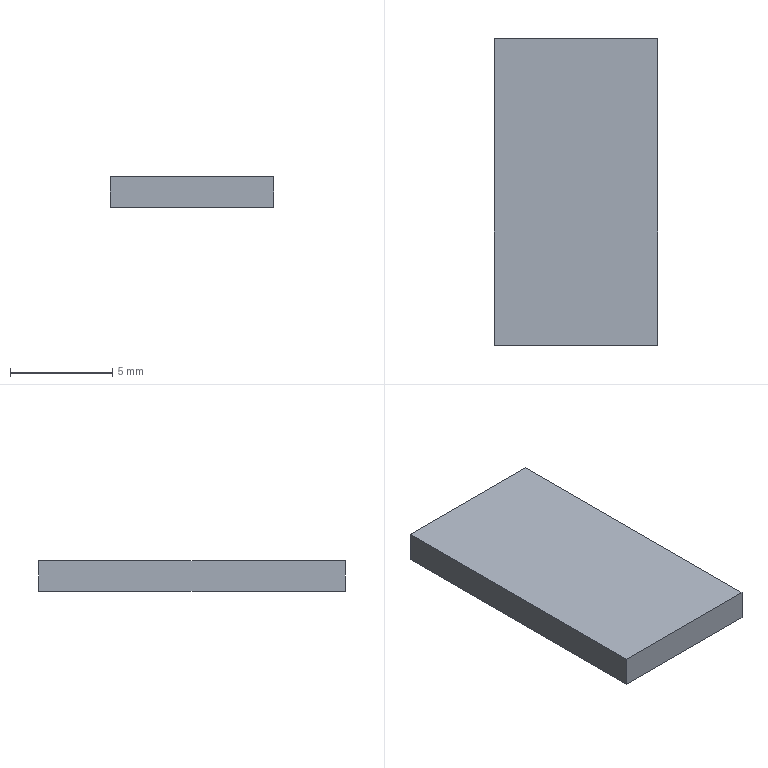Part | STEP file | T2x15x8 Rubber strip-dddeger_compressed | 1 solid | 6 faces | box 8 x 15 x 1.5 mm | volume 180 mm3 | plane 6
STEP:
#1=CARTESIAN_POINT('',(0.,0.,0.));
#2=DIRECTION('',(0.,0.,1.));
#3=DIRECTION('',(1.,0.,0.));
#4=AXIS2_PLACEMENT_3D('',#1,#2,#3);
#5=CARTESIAN_POINT('',(-629.155,-97.655,0.));
#6=VERTEX_POINT('',#5);
#7=CARTESIAN_POINT('',(-629.155,-82.655,0.));
#8=VERTEX_POINT('',#7);
#9=CARTESIAN_POINT('',(-629.155,-82.655,0.));
#10=DIRECTION('',(0.,1.,0.));
#11=VECTOR('',#10,1.);
#12=LINE('',#9,#11);
#13=CARTESIAN_POINT('',(-629.155,-82.655,1.5));
#14=DIRECTION('',(-1.,0.,0.));
#15=DIRECTION('',(0.,0.,1.));
#16=AXIS2_PLACEMENT_3D('',#13,#14,#15);
#17=PLANE('',#16);
#18=CARTESIAN_POINT('',(-1.5,0.));
#19=DIRECTION('',(0.,1.));
#20=VECTOR('',#19,1.);
#21=LINE('',#18,#20);
#22=(GEOMETRIC_REPRESENTATION_CONTEXT(2)PARAMETRIC_REPRESENTATION_CONTEXT()REPRESENTATION_CONTEXT('',''));
#23=DEFINITIONAL_REPRESENTATION('',(#21),#22);
#24=PCURVE('',#17,#23);
#25=CARTESIAN_POINT('',(0.,0.,0.));
#26=DIRECTION('',(0.,0.,-1.));
#27=DIRECTION('',(-1.,0.,0.));
#28=AXIS2_PLACEMENT_3D('',#25,#26,#27);
#29=PLANE('',#28);
#30=CARTESIAN_POINT('',(629.155,-82.655));
#31=DIRECTION('',(0.,1.));
#32=VECTOR('',#31,1.);
#33=LINE('',#30,#32);
#34=(GEOMETRIC_REPRESENTATION_CONTEXT(2)PARAMETRIC_REPRESENTATION_CONTEXT()REPRESENTATION_CONTEXT('',''));
#35=DEFINITIONAL_REPRESENTATION('',(#33),#34);
#36=PCURVE('',#29,#35);
#37=SURFACE_CURVE('',#12,(#24,#36),.PCURVE_S1.);
#38=EDGE_CURVE('',#6,#8,#37,.T.);
#39=ORIENTED_EDGE('',*,*,#38,.T.);
#40=CARTESIAN_POINT('',(-629.155,-82.655,1.5));
#41=VERTEX_POINT('',#40);
#42=CARTESIAN_POINT('',(-629.155,-82.655,1.5));
#43=DIRECTION('',(0.,0.,-1.));
#44=VECTOR('',#43,1.);
#45=LINE('',#42,#44);
#46=CARTESIAN_POINT('',(0.,0.));
#47=DIRECTION('',(-1.,0.));
#48=VECTOR('',#47,1.);
#49=LINE('',#46,#48);
#50=(GEOMETRIC_REPRESENTATION_CONTEXT(2)PARAMETRIC_REPRESENTATION_CONTEXT()REPRESENTATION_CONTEXT('',''));
#51=DEFINITIONAL_REPRESENTATION('',(#49),#50);
#52=PCURVE('',#17,#51);
#53=CARTESIAN_POINT('',(-629.155,-82.655,1.5));
#54=DIRECTION('',(0.,-1.,0.));
#55=DIRECTION('',(0.,0.,-1.));
#56=AXIS2_PLACEMENT_3D('',#53,#54,#55);
#57=PLANE('',#56);
#58=CARTESIAN_POINT('',(0.,0.));
#59=DIRECTION('',(1.,0.));
#60=VECTOR('',#59,1.);
#61=LINE('',#58,#60);
#62=(GEOMETRIC_REPRESENTATION_CONTEXT(2)PARAMETRIC_REPRESENTATION_CONTEXT()REPRESENTATION_CONTEXT('',''));
#63=DEFINITIONAL_REPRESENTATION('',(#61),#62);
#64=PCURVE('',#57,#63);
#65=SURFACE_CURVE('',#45,(#52,#64),.PCURVE_S1.);
#66=EDGE_CURVE('',#41,#8,#65,.T.);
#67=ORIENTED_EDGE('',*,*,#66,.F.);
#68=CARTESIAN_POINT('',(-629.155,-97.655,1.5));
#69=VERTEX_POINT('',#68);
#70=CARTESIAN_POINT('',(-629.155,-82.655,1.5));
#71=DIRECTION('',(0.,1.,0.));
#72=VECTOR('',#71,1.);
#73=LINE('',#70,#72);
#74=CARTESIAN_POINT('',(0.,0.));
#75=DIRECTION('',(0.,1.));
#76=VECTOR('',#75,1.);
#77=LINE('',#74,#76);
#78=(GEOMETRIC_REPRESENTATION_CONTEXT(2)PARAMETRIC_REPRESENTATION_CONTEXT()REPRESENTATION_CONTEXT('',''));
#79=DEFINITIONAL_REPRESENTATION('',(#77),#78);
#80=PCURVE('',#17,#79);
#81=CARTESIAN_POINT('',(0.,0.,1.5));
#82=DIRECTION('',(0.,0.,-1.));
#83=DIRECTION('',(-1.,0.,0.));
#84=AXIS2_PLACEMENT_3D('',#81,#82,#83);
#85=PLANE('',#84);
#86=CARTESIAN_POINT('',(629.155,-82.655));
#87=DIRECTION('',(0.,1.));
#88=VECTOR('',#87,1.);
#89=LINE('',#86,#88);
#90=(GEOMETRIC_REPRESENTATION_CONTEXT(2)PARAMETRIC_REPRESENTATION_CONTEXT()REPRESENTATION_CONTEXT('',''));
#91=DEFINITIONAL_REPRESENTATION('',(#89),#90);
#92=PCURVE('',#85,#91);
#93=SURFACE_CURVE('',#73,(#80,#92),.PCURVE_S1.);
#94=EDGE_CURVE('',#69,#41,#93,.T.);
#95=ORIENTED_EDGE('',*,*,#94,.F.);
#96=CARTESIAN_POINT('',(-629.155,-97.655,1.5));
#97=DIRECTION('',(0.,0.,-1.));
#98=VECTOR('',#97,1.);
#99=LINE('',#96,#98);
#100=CARTESIAN_POINT('',(0.,-15.));
#101=DIRECTION('',(-1.,0.));
#102=VECTOR('',#101,1.);
#103=LINE('',#100,#102);
#104=(GEOMETRIC_REPRESENTATION_CONTEXT(2)PARAMETRIC_REPRESENTATION_CONTEXT()REPRESENTATION_CONTEXT('',''));
#105=DEFINITIONAL_REPRESENTATION('',(#103),#104);
#106=PCURVE('',#17,#105);
#107=CARTESIAN_POINT('',(-629.155,-97.655,1.5));
#108=DIRECTION('',(0.,1.,0.));
#109=DIRECTION('',(0.,0.,1.));
#110=AXIS2_PLACEMENT_3D('',#107,#108,#109);
#111=PLANE('',#110);
#112=CARTESIAN_POINT('',(0.,0.));
#113=DIRECTION('',(-1.,0.));
#114=VECTOR('',#113,1.);
#115=LINE('',#112,#114);
#116=(GEOMETRIC_REPRESENTATION_CONTEXT(2)PARAMETRIC_REPRESENTATION_CONTEXT()REPRESENTATION_CONTEXT('',''));
#117=DEFINITIONAL_REPRESENTATION('',(#115),#116);
#118=PCURVE('',#111,#117);
#119=SURFACE_CURVE('',#99,(#106,#118),.PCURVE_S1.);
#120=EDGE_CURVE('',#69,#6,#119,.T.);
#121=ORIENTED_EDGE('',*,*,#120,.T.);
#122=EDGE_LOOP('',(#39,#67,#95,#121));
#123=FACE_BOUND('',#122,.T.);
#124=ADVANCED_FACE('',(#123),#17,.F.);
#125=CARTESIAN_POINT('',(-637.155,-82.655,0.));
#126=VERTEX_POINT('',#125);
#127=CARTESIAN_POINT('',(-629.155,-82.655,0.));
#128=DIRECTION('',(-1.,0.,0.));
#129=VECTOR('',#128,1.);
#130=LINE('',#127,#129);
#131=CARTESIAN_POINT('',(1.5,0.));
#132=DIRECTION('',(0.,-1.));
#133=VECTOR('',#132,1.);
#134=LINE('',#131,#133);
#135=(GEOMETRIC_REPRESENTATION_CONTEXT(2)PARAMETRIC_REPRESENTATION_CONTEXT()REPRESENTATION_CONTEXT('',''));
#136=DEFINITIONAL_REPRESENTATION('',(#134),#135);
#137=PCURVE('',#57,#136);
#138=CARTESIAN_POINT('',(629.155,-82.655));
#139=DIRECTION('',(1.,0.));
#140=VECTOR('',#139,1.);
#141=LINE('',#138,#140);
#142=(GEOMETRIC_REPRESENTATION_CONTEXT(2)PARAMETRIC_REPRESENTATION_CONTEXT()REPRESENTATION_CONTEXT('',''));
#143=DEFINITIONAL_REPRESENTATION('',(#141),#142);
#144=PCURVE('',#29,#143);
#145=SURFACE_CURVE('',#130,(#137,#144),.PCURVE_S1.);
#146=EDGE_CURVE('',#8,#126,#145,.T.);
#147=ORIENTED_EDGE('',*,*,#146,.T.);
#148=CARTESIAN_POINT('',(-637.155,-82.655,1.5));
#149=VERTEX_POINT('',#148);
#150=CARTESIAN_POINT('',(-637.155,-82.655,1.5));
#151=DIRECTION('',(0.,0.,-1.));
#152=VECTOR('',#151,1.);
#153=LINE('',#150,#152);
#154=CARTESIAN_POINT('',(0.,-8.));
#155=DIRECTION('',(1.,0.));
#156=VECTOR('',#155,1.);
#157=LINE('',#154,#156);
#158=(GEOMETRIC_REPRESENTATION_CONTEXT(2)PARAMETRIC_REPRESENTATION_CONTEXT()REPRESENTATION_CONTEXT('',''));
#159=DEFINITIONAL_REPRESENTATION('',(#157),#158);
#160=PCURVE('',#57,#159);
#161=CARTESIAN_POINT('',(-637.155,-82.655,1.5));
#162=DIRECTION('',(1.,0.,0.));
#163=DIRECTION('',(0.,0.,-1.));
#164=AXIS2_PLACEMENT_3D('',#161,#162,#163);
#165=PLANE('',#164);
#166=CARTESIAN_POINT('',(0.,0.));
#167=DIRECTION('',(1.,0.));
#168=VECTOR('',#167,1.);
#169=LINE('',#166,#168);
#170=(GEOMETRIC_REPRESENTATION_CONTEXT(2)PARAMETRIC_REPRESENTATION_CONTEXT()REPRESENTATION_CONTEXT('',''));
#171=DEFINITIONAL_REPRESENTATION('',(#169),#170);
#172=PCURVE('',#165,#171);
#173=SURFACE_CURVE('',#153,(#160,#172),.PCURVE_S1.);
#174=EDGE_CURVE('',#149,#126,#173,.T.);
#175=ORIENTED_EDGE('',*,*,#174,.F.);
#176=CARTESIAN_POINT('',(-629.155,-82.655,1.5));
#177=DIRECTION('',(-1.,0.,0.));
#178=VECTOR('',#177,1.);
#179=LINE('',#176,#178);
#180=CARTESIAN_POINT('',(0.,0.));
#181=DIRECTION('',(0.,-1.));
#182=VECTOR('',#181,1.);
#183=LINE('',#180,#182);
#184=(GEOMETRIC_REPRESENTATION_CONTEXT(2)PARAMETRIC_REPRESENTATION_CONTEXT()REPRESENTATION_CONTEXT('',''));
#185=DEFINITIONAL_REPRESENTATION('',(#183),#184);
#186=PCURVE('',#57,#185);
#187=CARTESIAN_POINT('',(629.155,-82.655));
#188=DIRECTION('',(1.,0.));
#189=VECTOR('',#188,1.);
#190=LINE('',#187,#189);
#191=(GEOMETRIC_REPRESENTATION_CONTEXT(2)PARAMETRIC_REPRESENTATION_CONTEXT()REPRESENTATION_CONTEXT('',''));
#192=DEFINITIONAL_REPRESENTATION('',(#190),#191);
#193=PCURVE('',#85,#192);
#194=SURFACE_CURVE('',#179,(#186,#193),.PCURVE_S1.);
#195=EDGE_CURVE('',#41,#149,#194,.T.);
#196=ORIENTED_EDGE('',*,*,#195,.F.);
#197=ORIENTED_EDGE('',*,*,#66,.T.);
#198=EDGE_LOOP('',(#147,#175,#196,#197));
#199=FACE_BOUND('',#198,.T.);
#200=ADVANCED_FACE('',(#199),#57,.F.);
#201=CARTESIAN_POINT('',(-637.155,-97.655,0.));
#202=VERTEX_POINT('',#201);
#203=CARTESIAN_POINT('',(-637.155,-82.655,0.));
#204=DIRECTION('',(0.,-1.,0.));
#205=VECTOR('',#204,1.);
#206=LINE('',#203,#205);
#207=CARTESIAN_POINT('',(1.5,0.));
#208=DIRECTION('',(0.,-1.));
#209=VECTOR('',#208,1.);
#210=LINE('',#207,#209);
#211=(GEOMETRIC_REPRESENTATION_CONTEXT(2)PARAMETRIC_REPRESENTATION_CONTEXT()REPRESENTATION_CONTEXT('',''));
#212=DEFINITIONAL_REPRESENTATION('',(#210),#211);
#213=PCURVE('',#165,#212);
#214=CARTESIAN_POINT('',(637.155,-82.655));
#215=DIRECTION('',(0.,-1.));
#216=VECTOR('',#215,1.);
#217=LINE('',#214,#216);
#218=(GEOMETRIC_REPRESENTATION_CONTEXT(2)PARAMETRIC_REPRESENTATION_CONTEXT()REPRESENTATION_CONTEXT('',''));
#219=DEFINITIONAL_REPRESENTATION('',(#217),#218);
#220=PCURVE('',#29,#219);
#221=SURFACE_CURVE('',#206,(#213,#220),.PCURVE_S1.);
#222=EDGE_CURVE('',#126,#202,#221,.T.);
#223=ORIENTED_EDGE('',*,*,#222,.T.);
#224=CARTESIAN_POINT('',(-637.155,-97.655,1.5));
#225=VERTEX_POINT('',#224);
#226=CARTESIAN_POINT('',(-637.155,-97.655,1.5));
#227=DIRECTION('',(0.,0.,-1.));
#228=VECTOR('',#227,1.);
#229=LINE('',#226,#228);
#230=CARTESIAN_POINT('',(0.,-15.));
#231=DIRECTION('',(1.,0.));
#232=VECTOR('',#231,1.);
#233=LINE('',#230,#232);
#234=(GEOMETRIC_REPRESENTATION_CONTEXT(2)PARAMETRIC_REPRESENTATION_CONTEXT()REPRESENTATION_CONTEXT('',''));
#235=DEFINITIONAL_REPRESENTATION('',(#233),#234);
#236=PCURVE('',#165,#235);
#237=CARTESIAN_POINT('',(0.,-8.));
#238=DIRECTION('',(-1.,0.));
#239=VECTOR('',#238,1.);
#240=LINE('',#237,#239);
#241=(GEOMETRIC_REPRESENTATION_CONTEXT(2)PARAMETRIC_REPRESENTATION_CONTEXT()REPRESENTATION_CONTEXT('',''));
#242=DEFINITIONAL_REPRESENTATION('',(#240),#241);
#243=PCURVE('',#111,#242);
#244=SURFACE_CURVE('',#229,(#236,#243),.PCURVE_S1.);
#245=EDGE_CURVE('',#225,#202,#244,.T.);
#246=ORIENTED_EDGE('',*,*,#245,.F.);
#247=CARTESIAN_POINT('',(-637.155,-82.655,1.5));
#248=DIRECTION('',(0.,-1.,0.));
#249=VECTOR('',#248,1.);
#250=LINE('',#247,#249);
#251=CARTESIAN_POINT('',(0.,0.));
#252=DIRECTION('',(0.,-1.));
#253=VECTOR('',#252,1.);
#254=LINE('',#251,#253);
#255=(GEOMETRIC_REPRESENTATION_CONTEXT(2)PARAMETRIC_REPRESENTATION_CONTEXT()REPRESENTATION_CONTEXT('',''));
#256=DEFINITIONAL_REPRESENTATION('',(#254),#255);
#257=PCURVE('',#165,#256);
#258=CARTESIAN_POINT('',(637.155,-82.655));
#259=DIRECTION('',(0.,-1.));
#260=VECTOR('',#259,1.);
#261=LINE('',#258,#260);
#262=(GEOMETRIC_REPRESENTATION_CONTEXT(2)PARAMETRIC_REPRESENTATION_CONTEXT()REPRESENTATION_CONTEXT('',''));
#263=DEFINITIONAL_REPRESENTATION('',(#261),#262);
#264=PCURVE('',#85,#263);
#265=SURFACE_CURVE('',#250,(#257,#264),.PCURVE_S1.);
#266=EDGE_CURVE('',#149,#225,#265,.T.);
#267=ORIENTED_EDGE('',*,*,#266,.F.);
#268=ORIENTED_EDGE('',*,*,#174,.T.);
#269=EDGE_LOOP('',(#223,#246,#267,#268));
#270=FACE_BOUND('',#269,.T.);
#271=ADVANCED_FACE('',(#270),#165,.F.);
#272=CARTESIAN_POINT('',(-629.155,-97.655,0.));
#273=DIRECTION('',(1.,0.,0.));
#274=VECTOR('',#273,1.);
#275=LINE('',#272,#274);
#276=CARTESIAN_POINT('',(-1.5,0.));
#277=DIRECTION('',(0.,1.));
#278=VECTOR('',#277,1.);
#279=LINE('',#276,#278);
#280=(GEOMETRIC_REPRESENTATION_CONTEXT(2)PARAMETRIC_REPRESENTATION_CONTEXT()REPRESENTATION_CONTEXT('',''));
#281=DEFINITIONAL_REPRESENTATION('',(#279),#280);
#282=PCURVE('',#111,#281);
#283=CARTESIAN_POINT('',(629.155,-97.655));
#284=DIRECTION('',(-1.,0.));
#285=VECTOR('',#284,1.);
#286=LINE('',#283,#285);
#287=(GEOMETRIC_REPRESENTATION_CONTEXT(2)PARAMETRIC_REPRESENTATION_CONTEXT()REPRESENTATION_CONTEXT('',''));
#288=DEFINITIONAL_REPRESENTATION('',(#286),#287);
#289=PCURVE('',#29,#288);
#290=SURFACE_CURVE('',#275,(#282,#289),.PCURVE_S1.);
#291=EDGE_CURVE('',#202,#6,#290,.T.);
#292=ORIENTED_EDGE('',*,*,#291,.T.);
#293=ORIENTED_EDGE('',*,*,#120,.F.);
#294=CARTESIAN_POINT('',(-629.155,-97.655,1.5));
#295=DIRECTION('',(1.,0.,0.));
#296=VECTOR('',#295,1.);
#297=LINE('',#294,#296);
#298=CARTESIAN_POINT('',(0.,0.));
#299=DIRECTION('',(0.,1.));
#300=VECTOR('',#299,1.);
#301=LINE('',#298,#300);
#302=(GEOMETRIC_REPRESENTATION_CONTEXT(2)PARAMETRIC_REPRESENTATION_CONTEXT()REPRESENTATION_CONTEXT('',''));
#303=DEFINITIONAL_REPRESENTATION('',(#301),#302);
#304=PCURVE('',#111,#303);
#305=CARTESIAN_POINT('',(629.155,-97.655));
#306=DIRECTION('',(-1.,0.));
#307=VECTOR('',#306,1.);
#308=LINE('',#305,#307);
#309=(GEOMETRIC_REPRESENTATION_CONTEXT(2)PARAMETRIC_REPRESENTATION_CONTEXT()REPRESENTATION_CONTEXT('',''));
#310=DEFINITIONAL_REPRESENTATION('',(#308),#309);
#311=PCURVE('',#85,#310);
#312=SURFACE_CURVE('',#297,(#304,#311),.PCURVE_S1.);
#313=EDGE_CURVE('',#225,#69,#312,.T.);
#314=ORIENTED_EDGE('',*,*,#313,.F.);
#315=ORIENTED_EDGE('',*,*,#245,.T.);
#316=EDGE_LOOP('',(#292,#293,#314,#315));
#317=FACE_BOUND('',#316,.T.);
#318=ADVANCED_FACE('',(#317),#111,.F.);
#319=ORIENTED_EDGE('',*,*,#94,.T.);
#320=ORIENTED_EDGE('',*,*,#195,.T.);
#321=ORIENTED_EDGE('',*,*,#266,.T.);
#322=ORIENTED_EDGE('',*,*,#313,.T.);
#323=EDGE_LOOP('',(#319,#320,#321,#322));
#324=FACE_BOUND('',#323,.T.);
#325=ADVANCED_FACE('',(#324),#85,.F.);
#326=ORIENTED_EDGE('',*,*,#38,.F.);
#327=ORIENTED_EDGE('',*,*,#291,.F.);
#328=ORIENTED_EDGE('',*,*,#222,.F.);
#329=ORIENTED_EDGE('',*,*,#146,.F.);
#330=EDGE_LOOP('',(#326,#327,#328,#329));
#331=FACE_BOUND('',#330,.T.);
#332=ADVANCED_FACE('',(#331),#29,.T.);
#333=CLOSED_SHELL('',(#124,#200,#271,#318,#325,#332));
#334=MANIFOLD_SOLID_BREP('',#333);
#335=(LENGTH_UNIT()NAMED_UNIT(*)SI_UNIT(.MILLI.,.METRE.));
#336=UNCERTAINTY_MEASURE_WITH_UNIT(LENGTH_MEASURE(0.0000001),#335,'','');
#337=(NAMED_UNIT(*)PLANE_ANGLE_UNIT()SI_UNIT($,.RADIAN.));
#338=(NAMED_UNIT(*)SI_UNIT($,.STERADIAN.)SOLID_ANGLE_UNIT());
#339=(GEOMETRIC_REPRESENTATION_CONTEXT(3)GLOBAL_UNCERTAINTY_ASSIGNED_CONTEXT((#336))GLOBAL_UNIT_ASSIGNED_CONTEXT((#335,#337,#338))REPRESENTATION_CONTEXT('',''));
#340=ADVANCED_BREP_SHAPE_REPRESENTATION('',(#4,#334),#339);